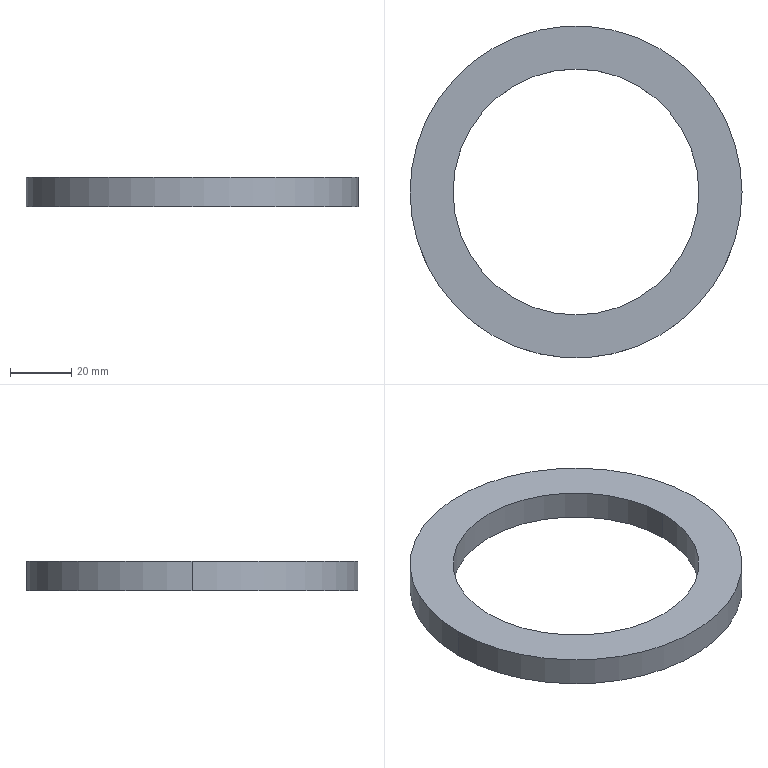Part | STEP file | 7016 Inner Spacer | 1 solid | 6 faces | box 108 x 108 x 9.5 mm | volume 39276 mm3 | cylinder 4 | plane 2 | commonest cylinder face diameters 80 x2 108 x2
STEP:
#1=CARTESIAN_POINT('',(40.,0.,9.5));
#2=VERTEX_POINT('',#1);
#3=CARTESIAN_POINT('',(-40.,0.,9.5));
#4=VERTEX_POINT('',#3);
#5=CARTESIAN_POINT('',(0.,0.,9.5));
#6=DIRECTION('',(0.,0.,-1.));
#7=DIRECTION('',(-1.,0.,0.));
#8=AXIS2_PLACEMENT_3D('',#5,#6,#7);
#9=CIRCLE('',#8,40.);
#10=EDGE_CURVE('',#2,#4,#9,.T.);
#11=ORIENTED_EDGE('',*,*,#10,.F.);
#12=CARTESIAN_POINT('',(40.,0.,0.));
#13=VERTEX_POINT('',#12);
#14=CARTESIAN_POINT('',(40.,0.,9.5));
#15=DIRECTION('',(0.,0.,-1.));
#16=VECTOR('',#15,1000.);
#17=LINE('',#14,#16);
#18=EDGE_CURVE('',#2,#13,#17,.T.);
#19=ORIENTED_EDGE('',*,*,#18,.T.);
#20=CARTESIAN_POINT('',(-40.,0.,0.));
#21=VERTEX_POINT('',#20);
#22=CARTESIAN_POINT('',(0.,0.,0.));
#23=DIRECTION('',(0.,0.,1.));
#24=DIRECTION('',(-1.,0.,0.));
#25=AXIS2_PLACEMENT_3D('',#22,#23,#24);
#26=CIRCLE('',#25,40.);
#27=EDGE_CURVE('',#21,#13,#26,.T.);
#28=ORIENTED_EDGE('',*,*,#27,.F.);
#29=CARTESIAN_POINT('',(-40.,0.,9.5));
#30=DIRECTION('',(0.,0.,-1.));
#31=VECTOR('',#30,1000.);
#32=LINE('',#29,#31);
#33=EDGE_CURVE('',#4,#21,#32,.T.);
#34=ORIENTED_EDGE('',*,*,#33,.F.);
#35=EDGE_LOOP('',(#11,#19,#28,#34));
#36=FACE_OUTER_BOUND('',#35,.T.);
#37=CARTESIAN_POINT('',(0.,0.,9.5));
#38=DIRECTION('',(0.,0.,-1.));
#39=DIRECTION('',(-1.,0.,0.));
#40=AXIS2_PLACEMENT_3D('',#37,#38,#39);
#41=CYLINDRICAL_SURFACE('',#40,40.);
#42=ADVANCED_FACE('',(#36),#41,.F.);
#43=CARTESIAN_POINT('',(54.,0.,9.5));
#44=VERTEX_POINT('',#43);
#45=CARTESIAN_POINT('',(-54.,0.,9.5));
#46=VERTEX_POINT('',#45);
#47=CARTESIAN_POINT('',(0.,0.,9.5));
#48=DIRECTION('',(0.,0.,1.));
#49=DIRECTION('',(-1.,0.,0.));
#50=AXIS2_PLACEMENT_3D('',#47,#48,#49);
#51=CIRCLE('',#50,54.);
#52=EDGE_CURVE('',#44,#46,#51,.T.);
#53=ORIENTED_EDGE('',*,*,#52,.F.);
#54=CARTESIAN_POINT('',(54.,0.,0.));
#55=VERTEX_POINT('',#54);
#56=CARTESIAN_POINT('',(54.,0.,9.5));
#57=DIRECTION('',(0.,0.,-1.));
#58=VECTOR('',#57,1000.);
#59=LINE('',#56,#58);
#60=EDGE_CURVE('',#44,#55,#59,.T.);
#61=ORIENTED_EDGE('',*,*,#60,.T.);
#62=CARTESIAN_POINT('',(-54.,0.,0.));
#63=VERTEX_POINT('',#62);
#64=CARTESIAN_POINT('',(0.,0.,0.));
#65=DIRECTION('',(0.,0.,1.));
#66=DIRECTION('',(-1.,0.,0.));
#67=AXIS2_PLACEMENT_3D('',#64,#65,#66);
#68=CIRCLE('',#67,54.);
#69=EDGE_CURVE('',#55,#63,#68,.T.);
#70=ORIENTED_EDGE('',*,*,#69,.T.);
#71=CARTESIAN_POINT('',(-54.,0.,9.5));
#72=DIRECTION('',(0.,0.,-1.));
#73=VECTOR('',#72,1000.);
#74=LINE('',#71,#73);
#75=EDGE_CURVE('',#46,#63,#74,.T.);
#76=ORIENTED_EDGE('',*,*,#75,.F.);
#77=EDGE_LOOP('',(#53,#61,#70,#76));
#78=FACE_OUTER_BOUND('',#77,.T.);
#79=CARTESIAN_POINT('',(0.,0.,9.5));
#80=DIRECTION('',(0.,0.,-1.));
#81=DIRECTION('',(-1.,0.,0.));
#82=AXIS2_PLACEMENT_3D('',#79,#80,#81);
#83=CYLINDRICAL_SURFACE('',#82,54.);
#84=ADVANCED_FACE('',(#78),#83,.T.);
#85=CARTESIAN_POINT('',(0.,0.,9.5));
#86=DIRECTION('',(0.,0.,-1.));
#87=DIRECTION('',(-1.,0.,0.));
#88=AXIS2_PLACEMENT_3D('',#85,#86,#87);
#89=CIRCLE('',#88,40.);
#90=EDGE_CURVE('',#4,#2,#89,.T.);
#91=ORIENTED_EDGE('',*,*,#90,.T.);
#92=ORIENTED_EDGE('',*,*,#10,.T.);
#93=EDGE_LOOP('',(#91,#92));
#94=FACE_BOUND('',#93,.T.);
#95=CARTESIAN_POINT('',(0.,0.,9.5));
#96=DIRECTION('',(0.,0.,1.));
#97=DIRECTION('',(-1.,0.,0.));
#98=AXIS2_PLACEMENT_3D('',#95,#96,#97);
#99=CIRCLE('',#98,54.);
#100=EDGE_CURVE('',#46,#44,#99,.T.);
#101=ORIENTED_EDGE('',*,*,#100,.T.);
#102=ORIENTED_EDGE('',*,*,#52,.T.);
#103=EDGE_LOOP('',(#101,#102));
#104=FACE_OUTER_BOUND('',#103,.T.);
#105=CARTESIAN_POINT('',(0.,0.,9.5));
#106=DIRECTION('',(0.,0.,1.));
#107=DIRECTION('',(1.,0.,0.));
#108=AXIS2_PLACEMENT_3D('',#105,#106,#107);
#109=PLANE('',#108);
#110=ADVANCED_FACE('',(#94,#104),#109,.T.);
#111=ORIENTED_EDGE('',*,*,#18,.F.);
#112=ORIENTED_EDGE('',*,*,#90,.F.);
#113=ORIENTED_EDGE('',*,*,#33,.T.);
#114=CARTESIAN_POINT('',(0.,0.,0.));
#115=DIRECTION('',(0.,0.,1.));
#116=DIRECTION('',(-1.,0.,0.));
#117=AXIS2_PLACEMENT_3D('',#114,#115,#116);
#118=CIRCLE('',#117,40.);
#119=EDGE_CURVE('',#13,#21,#118,.T.);
#120=ORIENTED_EDGE('',*,*,#119,.F.);
#121=EDGE_LOOP('',(#111,#112,#113,#120));
#122=FACE_OUTER_BOUND('',#121,.T.);
#123=CARTESIAN_POINT('',(0.,0.,9.5));
#124=DIRECTION('',(0.,0.,-1.));
#125=DIRECTION('',(-1.,0.,0.));
#126=AXIS2_PLACEMENT_3D('',#123,#124,#125);
#127=CYLINDRICAL_SURFACE('',#126,40.);
#128=ADVANCED_FACE('',(#122),#127,.F.);
#129=ORIENTED_EDGE('',*,*,#60,.F.);
#130=ORIENTED_EDGE('',*,*,#100,.F.);
#131=ORIENTED_EDGE('',*,*,#75,.T.);
#132=CARTESIAN_POINT('',(0.,0.,0.));
#133=DIRECTION('',(0.,0.,1.));
#134=DIRECTION('',(-1.,0.,0.));
#135=AXIS2_PLACEMENT_3D('',#132,#133,#134);
#136=CIRCLE('',#135,54.);
#137=EDGE_CURVE('',#63,#55,#136,.T.);
#138=ORIENTED_EDGE('',*,*,#137,.T.);
#139=EDGE_LOOP('',(#129,#130,#131,#138));
#140=FACE_OUTER_BOUND('',#139,.T.);
#141=CARTESIAN_POINT('',(0.,0.,9.5));
#142=DIRECTION('',(0.,0.,-1.));
#143=DIRECTION('',(-1.,0.,0.));
#144=AXIS2_PLACEMENT_3D('',#141,#142,#143);
#145=CYLINDRICAL_SURFACE('',#144,54.);
#146=ADVANCED_FACE('',(#140),#145,.T.);
#147=ORIENTED_EDGE('',*,*,#27,.T.);
#148=ORIENTED_EDGE('',*,*,#119,.T.);
#149=EDGE_LOOP('',(#147,#148));
#150=FACE_BOUND('',#149,.T.);
#151=ORIENTED_EDGE('',*,*,#137,.F.);
#152=ORIENTED_EDGE('',*,*,#69,.F.);
#153=EDGE_LOOP('',(#151,#152));
#154=FACE_OUTER_BOUND('',#153,.T.);
#155=CARTESIAN_POINT('',(0.,0.,0.));
#156=DIRECTION('',(0.,0.,1.));
#157=DIRECTION('',(1.,0.,0.));
#158=AXIS2_PLACEMENT_3D('',#155,#156,#157);
#159=PLANE('',#158);
#160=ADVANCED_FACE('',(#150,#154),#159,.F.);
#161=CLOSED_SHELL('',(#42,#84,#110,#128,#146,#160));
#162=MANIFOLD_SOLID_BREP('',#161);
#163=CARTESIAN_POINT('',(0.,0.,0.));
#164=DIRECTION('',(0.,0.,1.));
#165=DIRECTION('',(1.,0.,0.));
#166=AXIS2_PLACEMENT_3D('',#163,#164,#165);
#167=(LENGTH_UNIT()NAMED_UNIT(*)SI_UNIT(.MILLI.,.METRE.));
#168=UNCERTAINTY_MEASURE_WITH_UNIT(LENGTH_MEASURE(0.00001),#167,'','');
#169=(NAMED_UNIT(*)PLANE_ANGLE_UNIT()SI_UNIT($,.RADIAN.));
#170=(NAMED_UNIT(*)SI_UNIT($,.STERADIAN.)SOLID_ANGLE_UNIT());
#171=(GEOMETRIC_REPRESENTATION_CONTEXT(3)GLOBAL_UNCERTAINTY_ASSIGNED_CONTEXT((#168))GLOBAL_UNIT_ASSIGNED_CONTEXT((#167,#169,#170))REPRESENTATION_CONTEXT('',''));
#172=ADVANCED_BREP_SHAPE_REPRESENTATION('',(#162,#166),#171);